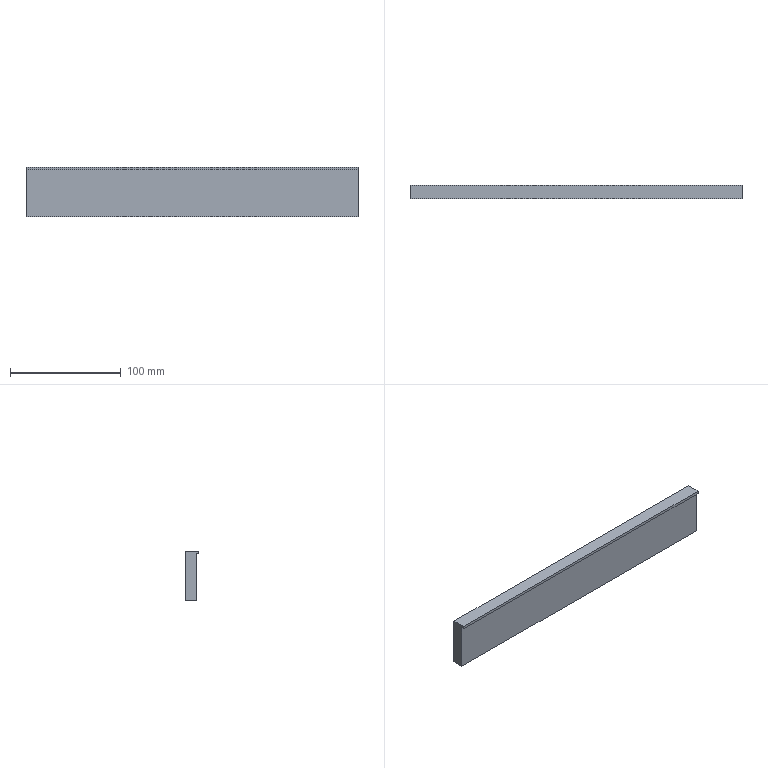Part | STEP file | Slider connecting plate | 1 solid | 8 faces | box 300 x 12 x 45 mm | volume 136500 mm3 | plane 8
STEP:
#1=CARTESIAN_POINT('',(150.,-32.,42.5));
#2=VERTEX_POINT('',#1);
#3=CARTESIAN_POINT('',(150.,-30.,42.5));
#4=VERTEX_POINT('',#3);
#5=CARTESIAN_POINT('',(150.,-32.,42.5));
#6=DIRECTION('',(0.,1.,0.));
#7=VECTOR('',#6,1000.);
#8=LINE('',#5,#7);
#9=EDGE_CURVE('',#2,#4,#8,.T.);
#10=ORIENTED_EDGE('',*,*,#9,.T.);
#11=CARTESIAN_POINT('',(150.,-30.,0.));
#12=VERTEX_POINT('',#11);
#13=CARTESIAN_POINT('',(150.,-30.,0.));
#14=DIRECTION('',(0.,0.,-1.));
#15=VECTOR('',#14,1000.);
#16=LINE('',#13,#15);
#17=EDGE_CURVE('',#4,#12,#16,.T.);
#18=ORIENTED_EDGE('',*,*,#17,.T.);
#19=CARTESIAN_POINT('',(150.,-20.,0.));
#20=VERTEX_POINT('',#19);
#21=CARTESIAN_POINT('',(150.,-20.,0.));
#22=DIRECTION('',(0.,1.,0.));
#23=VECTOR('',#22,1000.);
#24=LINE('',#21,#23);
#25=EDGE_CURVE('',#12,#20,#24,.T.);
#26=ORIENTED_EDGE('',*,*,#25,.T.);
#27=CARTESIAN_POINT('',(150.,-20.,45.));
#28=VERTEX_POINT('',#27);
#29=CARTESIAN_POINT('',(150.,-20.,45.));
#30=DIRECTION('',(0.,0.,-1.));
#31=VECTOR('',#30,1000.);
#32=LINE('',#29,#31);
#33=EDGE_CURVE('',#28,#20,#32,.T.);
#34=ORIENTED_EDGE('',*,*,#33,.F.);
#35=CARTESIAN_POINT('',(150.,-32.,45.));
#36=VERTEX_POINT('',#35);
#37=CARTESIAN_POINT('',(150.,-20.,45.));
#38=DIRECTION('',(0.,1.,0.));
#39=VECTOR('',#38,1000.);
#40=LINE('',#37,#39);
#41=EDGE_CURVE('',#36,#28,#40,.T.);
#42=ORIENTED_EDGE('',*,*,#41,.F.);
#43=CARTESIAN_POINT('',(150.,-32.,45.));
#44=DIRECTION('',(0.,0.,-1.));
#45=VECTOR('',#44,1000.);
#46=LINE('',#43,#45);
#47=EDGE_CURVE('',#36,#2,#46,.T.);
#48=ORIENTED_EDGE('',*,*,#47,.T.);
#49=EDGE_LOOP('',(#10,#18,#26,#34,#42,#48));
#50=FACE_OUTER_BOUND('',#49,.T.);
#51=CARTESIAN_POINT('',(150.,-20.,45.));
#52=DIRECTION('',(-1.,0.,0.));
#53=DIRECTION('',(0.,0.,1.));
#54=AXIS2_PLACEMENT_3D('',#51,#52,#53);
#55=PLANE('',#54);
#56=ADVANCED_FACE('',(#50),#55,.F.);
#57=CARTESIAN_POINT('',(-150.,-20.,0.));
#58=VERTEX_POINT('',#57);
#59=CARTESIAN_POINT('',(150.,-20.,0.));
#60=DIRECTION('',(-1.,0.,0.));
#61=VECTOR('',#60,1000.);
#62=LINE('',#59,#61);
#63=EDGE_CURVE('',#20,#58,#62,.T.);
#64=ORIENTED_EDGE('',*,*,#63,.T.);
#65=CARTESIAN_POINT('',(-150.,-20.,45.));
#66=VERTEX_POINT('',#65);
#67=CARTESIAN_POINT('',(-150.,-20.,45.));
#68=DIRECTION('',(0.,0.,-1.));
#69=VECTOR('',#68,1000.);
#70=LINE('',#67,#69);
#71=EDGE_CURVE('',#66,#58,#70,.T.);
#72=ORIENTED_EDGE('',*,*,#71,.F.);
#73=CARTESIAN_POINT('',(150.,-20.,45.));
#74=DIRECTION('',(-1.,0.,0.));
#75=VECTOR('',#74,1000.);
#76=LINE('',#73,#75);
#77=EDGE_CURVE('',#28,#66,#76,.T.);
#78=ORIENTED_EDGE('',*,*,#77,.F.);
#79=ORIENTED_EDGE('',*,*,#33,.T.);
#80=EDGE_LOOP('',(#64,#72,#78,#79));
#81=FACE_OUTER_BOUND('',#80,.T.);
#82=CARTESIAN_POINT('',(150.,-20.,45.));
#83=DIRECTION('',(0.,-1.,0.));
#84=DIRECTION('',(0.,0.,-1.));
#85=AXIS2_PLACEMENT_3D('',#82,#83,#84);
#86=PLANE('',#85);
#87=ADVANCED_FACE('',(#81),#86,.F.);
#88=CARTESIAN_POINT('',(-150.,-30.,0.));
#89=VERTEX_POINT('',#88);
#90=CARTESIAN_POINT('',(-150.,-20.,0.));
#91=DIRECTION('',(0.,-1.,0.));
#92=VECTOR('',#91,1000.);
#93=LINE('',#90,#92);
#94=EDGE_CURVE('',#58,#89,#93,.T.);
#95=ORIENTED_EDGE('',*,*,#94,.T.);
#96=CARTESIAN_POINT('',(-150.,-30.,42.5));
#97=VERTEX_POINT('',#96);
#98=CARTESIAN_POINT('',(-150.,-30.,0.));
#99=DIRECTION('',(0.,0.,-1.));
#100=VECTOR('',#99,1000.);
#101=LINE('',#98,#100);
#102=EDGE_CURVE('',#97,#89,#101,.T.);
#103=ORIENTED_EDGE('',*,*,#102,.F.);
#104=CARTESIAN_POINT('',(-150.,-32.,42.5));
#105=VERTEX_POINT('',#104);
#106=CARTESIAN_POINT('',(-150.,-32.,42.5));
#107=DIRECTION('',(0.,1.,0.));
#108=VECTOR('',#107,1000.);
#109=LINE('',#106,#108);
#110=EDGE_CURVE('',#105,#97,#109,.T.);
#111=ORIENTED_EDGE('',*,*,#110,.F.);
#112=CARTESIAN_POINT('',(-150.,-32.,45.));
#113=VERTEX_POINT('',#112);
#114=CARTESIAN_POINT('',(-150.,-32.,45.));
#115=DIRECTION('',(0.,0.,-1.));
#116=VECTOR('',#115,1000.);
#117=LINE('',#114,#116);
#118=EDGE_CURVE('',#113,#105,#117,.T.);
#119=ORIENTED_EDGE('',*,*,#118,.F.);
#120=CARTESIAN_POINT('',(-150.,-20.,45.));
#121=DIRECTION('',(0.,-1.,0.));
#122=VECTOR('',#121,1000.);
#123=LINE('',#120,#122);
#124=EDGE_CURVE('',#66,#113,#123,.T.);
#125=ORIENTED_EDGE('',*,*,#124,.F.);
#126=ORIENTED_EDGE('',*,*,#71,.T.);
#127=EDGE_LOOP('',(#95,#103,#111,#119,#125,#126));
#128=FACE_OUTER_BOUND('',#127,.T.);
#129=CARTESIAN_POINT('',(-150.,-20.,45.));
#130=DIRECTION('',(1.,0.,0.));
#131=DIRECTION('',(0.,0.,-1.));
#132=AXIS2_PLACEMENT_3D('',#129,#130,#131);
#133=PLANE('',#132);
#134=ADVANCED_FACE('',(#128),#133,.F.);
#135=ORIENTED_EDGE('',*,*,#118,.T.);
#136=CARTESIAN_POINT('',(150.,-32.,42.5));
#137=DIRECTION('',(-1.,0.,0.));
#138=VECTOR('',#137,1000.);
#139=LINE('',#136,#138);
#140=EDGE_CURVE('',#2,#105,#139,.T.);
#141=ORIENTED_EDGE('',*,*,#140,.F.);
#142=ORIENTED_EDGE('',*,*,#47,.F.);
#143=CARTESIAN_POINT('',(150.,-32.,45.));
#144=DIRECTION('',(1.,0.,0.));
#145=VECTOR('',#144,1000.);
#146=LINE('',#143,#145);
#147=EDGE_CURVE('',#113,#36,#146,.T.);
#148=ORIENTED_EDGE('',*,*,#147,.F.);
#149=EDGE_LOOP('',(#135,#141,#142,#148));
#150=FACE_OUTER_BOUND('',#149,.T.);
#151=CARTESIAN_POINT('',(150.,-32.,45.));
#152=DIRECTION('',(0.,1.,0.));
#153=DIRECTION('',(-1.,0.,0.));
#154=AXIS2_PLACEMENT_3D('',#151,#152,#153);
#155=PLANE('',#154);
#156=ADVANCED_FACE('',(#150),#155,.F.);
#157=ORIENTED_EDGE('',*,*,#41,.T.);
#158=ORIENTED_EDGE('',*,*,#77,.T.);
#159=ORIENTED_EDGE('',*,*,#124,.T.);
#160=ORIENTED_EDGE('',*,*,#147,.T.);
#161=EDGE_LOOP('',(#157,#158,#159,#160));
#162=FACE_OUTER_BOUND('',#161,.T.);
#163=CARTESIAN_POINT('',(0.,0.,45.));
#164=DIRECTION('',(0.,0.,-1.));
#165=DIRECTION('',(-1.,0.,0.));
#166=AXIS2_PLACEMENT_3D('',#163,#164,#165);
#167=PLANE('',#166);
#168=ADVANCED_FACE('',(#162),#167,.F.);
#169=CARTESIAN_POINT('',(150.,-30.,0.));
#170=DIRECTION('',(-1.,0.,0.));
#171=VECTOR('',#170,1000.);
#172=LINE('',#169,#171);
#173=EDGE_CURVE('',#12,#89,#172,.T.);
#174=ORIENTED_EDGE('',*,*,#173,.T.);
#175=ORIENTED_EDGE('',*,*,#94,.F.);
#176=ORIENTED_EDGE('',*,*,#63,.F.);
#177=ORIENTED_EDGE('',*,*,#25,.F.);
#178=EDGE_LOOP('',(#174,#175,#176,#177));
#179=FACE_OUTER_BOUND('',#178,.T.);
#180=CARTESIAN_POINT('',(0.,0.,0.));
#181=DIRECTION('',(0.,0.,-1.));
#182=DIRECTION('',(-1.,0.,0.));
#183=AXIS2_PLACEMENT_3D('',#180,#181,#182);
#184=PLANE('',#183);
#185=ADVANCED_FACE('',(#179),#184,.T.);
#186=ORIENTED_EDGE('',*,*,#102,.T.);
#187=ORIENTED_EDGE('',*,*,#173,.F.);
#188=ORIENTED_EDGE('',*,*,#17,.F.);
#189=CARTESIAN_POINT('',(150.,-30.,42.5));
#190=DIRECTION('',(-1.,0.,0.));
#191=VECTOR('',#190,1000.);
#192=LINE('',#189,#191);
#193=EDGE_CURVE('',#4,#97,#192,.T.);
#194=ORIENTED_EDGE('',*,*,#193,.T.);
#195=EDGE_LOOP('',(#186,#187,#188,#194));
#196=FACE_OUTER_BOUND('',#195,.T.);
#197=CARTESIAN_POINT('',(150.,-30.,0.));
#198=DIRECTION('',(0.,1.,0.));
#199=DIRECTION('',(0.,0.,1.));
#200=AXIS2_PLACEMENT_3D('',#197,#198,#199);
#201=PLANE('',#200);
#202=ADVANCED_FACE('',(#196),#201,.F.);
#203=ORIENTED_EDGE('',*,*,#110,.T.);
#204=ORIENTED_EDGE('',*,*,#193,.F.);
#205=ORIENTED_EDGE('',*,*,#9,.F.);
#206=ORIENTED_EDGE('',*,*,#140,.T.);
#207=EDGE_LOOP('',(#203,#204,#205,#206));
#208=FACE_OUTER_BOUND('',#207,.T.);
#209=CARTESIAN_POINT('',(150.,-32.,42.5));
#210=DIRECTION('',(0.,0.,1.));
#211=DIRECTION('',(1.,0.,0.));
#212=AXIS2_PLACEMENT_3D('',#209,#210,#211);
#213=PLANE('',#212);
#214=ADVANCED_FACE('',(#208),#213,.F.);
#215=CLOSED_SHELL('',(#56,#87,#134,#156,#168,#185,#202,#214));
#216=MANIFOLD_SOLID_BREP('',#215);
#217=CARTESIAN_POINT('',(0.,0.,0.));
#218=DIRECTION('',(0.,0.,1.));
#219=DIRECTION('',(1.,0.,0.));
#220=AXIS2_PLACEMENT_3D('',#217,#218,#219);
#221=(LENGTH_UNIT()NAMED_UNIT(*)SI_UNIT(.MILLI.,.METRE.));
#222=UNCERTAINTY_MEASURE_WITH_UNIT(LENGTH_MEASURE(0.00001),#221,'','');
#223=(NAMED_UNIT(*)PLANE_ANGLE_UNIT()SI_UNIT($,.RADIAN.));
#224=(NAMED_UNIT(*)SI_UNIT($,.STERADIAN.)SOLID_ANGLE_UNIT());
#225=(GEOMETRIC_REPRESENTATION_CONTEXT(3)GLOBAL_UNCERTAINTY_ASSIGNED_CONTEXT((#222))GLOBAL_UNIT_ASSIGNED_CONTEXT((#221,#223,#224))REPRESENTATION_CONTEXT('',''));
#226=ADVANCED_BREP_SHAPE_REPRESENTATION('',(#216,#220),#225);